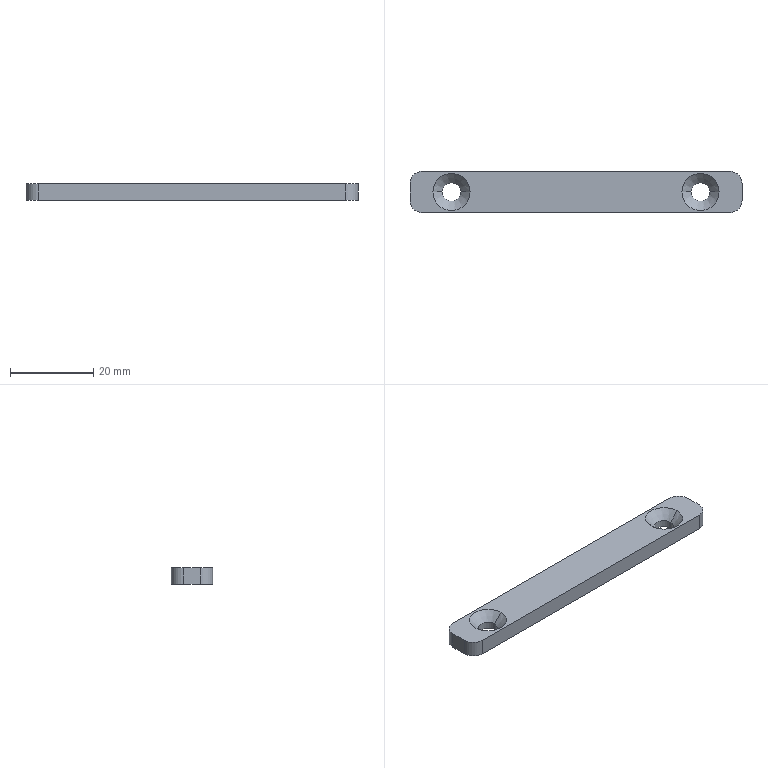Part | STEP file | Belt support strip | 1 solid | 18 faces | box 80 x 10 x 4 mm | volume 2948 mm3 | cylinder 8 | plane 6 | cone 4 | commonest cylinder face diameters 4.5 x4 6 x4
STEP:
#1=CARTESIAN_POINT('',(0.,0.,0.));
#2=DIRECTION('',(0.,0.,1.));
#3=DIRECTION('',(1.,0.,0.));
#4=AXIS2_PLACEMENT_3D('',#1,#2,#3);
#5=CARTESIAN_POINT('',(-116.718,13.068,1.77));
#6=VERTEX_POINT('',#5);
#7=CARTESIAN_POINT('',(-114.488,13.068,4.));
#8=VERTEX_POINT('',#7);
#9=CARTESIAN_POINT('',(-114.488,13.068,4.));
#10=DIRECTION('',(0.7071,0.,0.7071));
#11=VECTOR('',#10,1.);
#12=LINE('',#9,#11);
#13=CARTESIAN_POINT('',(-118.968,13.068,4.));
#14=DIRECTION('',(0.,0.,1.));
#15=DIRECTION('',(1.,0.,0.));
#16=AXIS2_PLACEMENT_3D('',#13,#14,#15);
#17=CONICAL_SURFACE('',#16,4.48,0.7854);
#18=CARTESIAN_POINT('',(6.283,0.));
#19=DIRECTION('',(0.,1.));
#20=VECTOR('',#19,1.);
#21=LINE('',#18,#20);
#22=(GEOMETRIC_REPRESENTATION_CONTEXT(2)PARAMETRIC_REPRESENTATION_CONTEXT()REPRESENTATION_CONTEXT('',''));
#23=DEFINITIONAL_REPRESENTATION('',(#21),#22);
#24=PCURVE('',#17,#23);
#25=CARTESIAN_POINT('',(-118.968,13.068,4.));
#26=DIRECTION('',(0.,0.,1.));
#27=DIRECTION('',(1.,0.,0.));
#28=AXIS2_PLACEMENT_3D('',#25,#26,#27);
#29=CONICAL_SURFACE('',#28,4.48,0.7854);
#30=CARTESIAN_POINT('',(0.,0.));
#31=DIRECTION('',(0.,1.));
#32=VECTOR('',#31,1.);
#33=LINE('',#30,#32);
#34=(GEOMETRIC_REPRESENTATION_CONTEXT(2)PARAMETRIC_REPRESENTATION_CONTEXT()REPRESENTATION_CONTEXT('',''));
#35=DEFINITIONAL_REPRESENTATION('',(#33),#34);
#36=PCURVE('',#29,#35);
#37=SURFACE_CURVE('',#12,(#24,#36),.PCURVE_S1.);
#38=EDGE_CURVE('',#6,#8,#37,.T.);
#39=ORIENTED_EDGE('',*,*,#38,.T.);
#40=CARTESIAN_POINT('',(-123.448,13.068,4.));
#41=VERTEX_POINT('',#40);
#42=CARTESIAN_POINT('',(-118.968,13.068,4.));
#43=DIRECTION('',(0.,0.,1.));
#44=DIRECTION('',(1.,0.,0.));
#45=AXIS2_PLACEMENT_3D('',#42,#43,#44);
#46=CIRCLE('',#45,4.48);
#47=CARTESIAN_POINT('',(0.,0.));
#48=DIRECTION('',(1.,0.));
#49=VECTOR('',#48,1.);
#50=LINE('',#47,#49);
#51=(GEOMETRIC_REPRESENTATION_CONTEXT(2)PARAMETRIC_REPRESENTATION_CONTEXT()REPRESENTATION_CONTEXT('',''));
#52=DEFINITIONAL_REPRESENTATION('',(#50),#51);
#53=PCURVE('',#17,#52);
#54=CARTESIAN_POINT('',(-51.968,15.068,4.));
#55=DIRECTION('',(0.,0.,-1.));
#56=DIRECTION('',(-1.,0.,0.));
#57=AXIS2_PLACEMENT_3D('',#54,#55,#56);
#58=PLANE('',#57);
#59=CARTESIAN_POINT('',(62.52,-2.));
#60=CARTESIAN_POINT('',(62.52,5.76));
#61=CARTESIAN_POINT('',(69.24,1.88));
#62=CARTESIAN_POINT('',(75.96,-2.));
#63=CARTESIAN_POINT('',(69.24,-5.88));
#64=CARTESIAN_POINT('',(62.52,-9.76));
#65=CARTESIAN_POINT('',(62.52,-2.));
#66=(BOUNDED_CURVE()B_SPLINE_CURVE(2,(#59,#60,#61,#62,#63,#64,#65),.UNSPECIFIED.,.T.,.F.)B_SPLINE_CURVE_WITH_KNOTS((1,2,2,2,2,1),(-2.094,0.,2.094,4.189,6.283,8.378),.UNSPECIFIED.)CURVE()GEOMETRIC_REPRESENTATION_ITEM()RATIONAL_B_SPLINE_CURVE((1.,0.5,1.,0.5,1.,0.5,1.))REPRESENTATION_ITEM(''));
#67=(GEOMETRIC_REPRESENTATION_CONTEXT(2)PARAMETRIC_REPRESENTATION_CONTEXT()REPRESENTATION_CONTEXT('',''));
#68=DEFINITIONAL_REPRESENTATION('',(#66),#67);
#69=PCURVE('',#58,#68);
#70=SURFACE_CURVE('',#46,(#53,#69),.PCURVE_S1.);
#71=EDGE_CURVE('',#41,#8,#70,.T.);
#72=ORIENTED_EDGE('',*,*,#71,.F.);
#73=CARTESIAN_POINT('',(-121.218,13.068,1.77));
#74=VERTEX_POINT('',#73);
#75=CARTESIAN_POINT('',(-123.448,13.068,4.));
#76=DIRECTION('',(-0.7071,0.,0.7071));
#77=VECTOR('',#76,1.);
#78=LINE('',#75,#77);
#79=CARTESIAN_POINT('',(3.142,0.));
#80=DIRECTION('',(0.,1.));
#81=VECTOR('',#80,1.);
#82=LINE('',#79,#81);
#83=(GEOMETRIC_REPRESENTATION_CONTEXT(2)PARAMETRIC_REPRESENTATION_CONTEXT()REPRESENTATION_CONTEXT('',''));
#84=DEFINITIONAL_REPRESENTATION('',(#82),#83);
#85=PCURVE('',#17,#84);
#86=CARTESIAN_POINT('',(3.142,0.));
#87=DIRECTION('',(0.,1.));
#88=VECTOR('',#87,1.);
#89=LINE('',#86,#88);
#90=(GEOMETRIC_REPRESENTATION_CONTEXT(2)PARAMETRIC_REPRESENTATION_CONTEXT()REPRESENTATION_CONTEXT('',''));
#91=DEFINITIONAL_REPRESENTATION('',(#89),#90);
#92=PCURVE('',#29,#91);
#93=SURFACE_CURVE('',#78,(#85,#92),.PCURVE_S1.);
#94=EDGE_CURVE('',#74,#41,#93,.T.);
#95=ORIENTED_EDGE('',*,*,#94,.F.);
#96=CARTESIAN_POINT('',(-118.968,13.068,1.77));
#97=DIRECTION('',(0.,0.,1.));
#98=DIRECTION('',(1.,0.,0.));
#99=AXIS2_PLACEMENT_3D('',#96,#97,#98);
#100=CIRCLE('',#99,2.25);
#101=CARTESIAN_POINT('',(0.,-2.23));
#102=DIRECTION('',(1.,0.));
#103=VECTOR('',#102,1.);
#104=LINE('',#101,#103);
#105=(GEOMETRIC_REPRESENTATION_CONTEXT(2)PARAMETRIC_REPRESENTATION_CONTEXT()REPRESENTATION_CONTEXT('',''));
#106=DEFINITIONAL_REPRESENTATION('',(#104),#105);
#107=PCURVE('',#17,#106);
#108=CARTESIAN_POINT('',(-118.968,13.068,4.));
#109=DIRECTION('',(0.,0.,1.));
#110=DIRECTION('',(1.,0.,0.));
#111=AXIS2_PLACEMENT_3D('',#108,#109,#110);
#112=CYLINDRICAL_SURFACE('',#111,2.25);
#113=CARTESIAN_POINT('',(0.,-2.23));
#114=DIRECTION('',(1.,0.));
#115=VECTOR('',#114,1.);
#116=LINE('',#113,#115);
#117=(GEOMETRIC_REPRESENTATION_CONTEXT(2)PARAMETRIC_REPRESENTATION_CONTEXT()REPRESENTATION_CONTEXT('',''));
#118=DEFINITIONAL_REPRESENTATION('',(#116),#117);
#119=PCURVE('',#112,#118);
#120=SURFACE_CURVE('',#100,(#107,#119),.PCURVE_S1.);
#121=EDGE_CURVE('',#74,#6,#120,.T.);
#122=ORIENTED_EDGE('',*,*,#121,.T.);
#123=EDGE_LOOP('',(#39,#72,#95,#122));
#124=FACE_BOUND('',#123,.F.);
#125=ADVANCED_FACE('',(#124),#17,.F.);
#126=CARTESIAN_POINT('',(-116.718,13.068,0.));
#127=VERTEX_POINT('',#126);
#128=CARTESIAN_POINT('',(-116.718,13.068,4.));
#129=DIRECTION('',(0.,0.,1.));
#130=VECTOR('',#129,1.);
#131=LINE('',#128,#130);
#132=CARTESIAN_POINT('',(6.283,0.));
#133=DIRECTION('',(0.,1.));
#134=VECTOR('',#133,1.);
#135=LINE('',#132,#134);
#136=(GEOMETRIC_REPRESENTATION_CONTEXT(2)PARAMETRIC_REPRESENTATION_CONTEXT()REPRESENTATION_CONTEXT('',''));
#137=DEFINITIONAL_REPRESENTATION('',(#135),#136);
#138=PCURVE('',#112,#137);
#139=CARTESIAN_POINT('',(-118.968,13.068,4.));
#140=DIRECTION('',(0.,0.,1.));
#141=DIRECTION('',(1.,0.,0.));
#142=AXIS2_PLACEMENT_3D('',#139,#140,#141);
#143=CYLINDRICAL_SURFACE('',#142,2.25);
#144=CARTESIAN_POINT('',(0.,0.));
#145=DIRECTION('',(0.,1.));
#146=VECTOR('',#145,1.);
#147=LINE('',#144,#146);
#148=(GEOMETRIC_REPRESENTATION_CONTEXT(2)PARAMETRIC_REPRESENTATION_CONTEXT()REPRESENTATION_CONTEXT('',''));
#149=DEFINITIONAL_REPRESENTATION('',(#147),#148);
#150=PCURVE('',#143,#149);
#151=SURFACE_CURVE('',#131,(#138,#150),.PCURVE_S1.);
#152=EDGE_CURVE('',#127,#6,#151,.T.);
#153=ORIENTED_EDGE('',*,*,#152,.T.);
#154=ORIENTED_EDGE('',*,*,#121,.F.);
#155=CARTESIAN_POINT('',(-121.218,13.068,0.));
#156=VERTEX_POINT('',#155);
#157=CARTESIAN_POINT('',(-121.218,13.068,4.));
#158=DIRECTION('',(0.,0.,1.));
#159=VECTOR('',#158,1.);
#160=LINE('',#157,#159);
#161=CARTESIAN_POINT('',(3.142,0.));
#162=DIRECTION('',(0.,1.));
#163=VECTOR('',#162,1.);
#164=LINE('',#161,#163);
#165=(GEOMETRIC_REPRESENTATION_CONTEXT(2)PARAMETRIC_REPRESENTATION_CONTEXT()REPRESENTATION_CONTEXT('',''));
#166=DEFINITIONAL_REPRESENTATION('',(#164),#165);
#167=PCURVE('',#112,#166);
#168=CARTESIAN_POINT('',(3.142,0.));
#169=DIRECTION('',(0.,1.));
#170=VECTOR('',#169,1.);
#171=LINE('',#168,#170);
#172=(GEOMETRIC_REPRESENTATION_CONTEXT(2)PARAMETRIC_REPRESENTATION_CONTEXT()REPRESENTATION_CONTEXT('',''));
#173=DEFINITIONAL_REPRESENTATION('',(#171),#172);
#174=PCURVE('',#143,#173);
#175=SURFACE_CURVE('',#160,(#167,#174),.PCURVE_S1.);
#176=EDGE_CURVE('',#156,#74,#175,.T.);
#177=ORIENTED_EDGE('',*,*,#176,.F.);
#178=CARTESIAN_POINT('',(-118.968,13.068,0.));
#179=DIRECTION('',(0.,0.,1.));
#180=DIRECTION('',(1.,0.,0.));
#181=AXIS2_PLACEMENT_3D('',#178,#179,#180);
#182=CIRCLE('',#181,2.25);
#183=CARTESIAN_POINT('',(0.,-4.));
#184=DIRECTION('',(1.,0.));
#185=VECTOR('',#184,1.);
#186=LINE('',#183,#185);
#187=(GEOMETRIC_REPRESENTATION_CONTEXT(2)PARAMETRIC_REPRESENTATION_CONTEXT()REPRESENTATION_CONTEXT('',''));
#188=DEFINITIONAL_REPRESENTATION('',(#186),#187);
#189=PCURVE('',#112,#188);
#190=CARTESIAN_POINT('',(-51.968,15.068,0.));
#191=DIRECTION('',(0.,0.,-1.));
#192=DIRECTION('',(-1.,0.,0.));
#193=AXIS2_PLACEMENT_3D('',#190,#191,#192);
#194=PLANE('',#193);
#195=CARTESIAN_POINT('',(64.75,-2.));
#196=CARTESIAN_POINT('',(64.75,1.897));
#197=CARTESIAN_POINT('',(68.125,-0.05144));
#198=CARTESIAN_POINT('',(71.5,-2.));
#199=CARTESIAN_POINT('',(68.125,-3.949));
#200=CARTESIAN_POINT('',(64.75,-5.897));
#201=CARTESIAN_POINT('',(64.75,-2.));
#202=(BOUNDED_CURVE()B_SPLINE_CURVE(2,(#195,#196,#197,#198,#199,#200,#201),.UNSPECIFIED.,.T.,.F.)B_SPLINE_CURVE_WITH_KNOTS((1,2,2,2,2,1),(-2.094,0.,2.094,4.189,6.283,8.378),.UNSPECIFIED.)CURVE()GEOMETRIC_REPRESENTATION_ITEM()RATIONAL_B_SPLINE_CURVE((1.,0.5,1.,0.5,1.,0.5,1.))REPRESENTATION_ITEM(''));
#203=(GEOMETRIC_REPRESENTATION_CONTEXT(2)PARAMETRIC_REPRESENTATION_CONTEXT()REPRESENTATION_CONTEXT('',''));
#204=DEFINITIONAL_REPRESENTATION('',(#202),#203);
#205=PCURVE('',#194,#204);
#206=SURFACE_CURVE('',#182,(#189,#205),.PCURVE_S1.);
#207=EDGE_CURVE('',#156,#127,#206,.T.);
#208=ORIENTED_EDGE('',*,*,#207,.T.);
#209=EDGE_LOOP('',(#153,#154,#177,#208));
#210=FACE_BOUND('',#209,.F.);
#211=ADVANCED_FACE('',(#210),#112,.F.);
#212=CARTESIAN_POINT('',(-56.718,13.068,1.77));
#213=VERTEX_POINT('',#212);
#214=CARTESIAN_POINT('',(-54.488,13.068,4.));
#215=VERTEX_POINT('',#214);
#216=CARTESIAN_POINT('',(-54.488,13.068,4.));
#217=DIRECTION('',(0.7071,0.,0.7071));
#218=VECTOR('',#217,1.);
#219=LINE('',#216,#218);
#220=CARTESIAN_POINT('',(-58.968,13.068,4.));
#221=DIRECTION('',(0.,0.,1.));
#222=DIRECTION('',(1.,0.,0.));
#223=AXIS2_PLACEMENT_3D('',#220,#221,#222);
#224=CONICAL_SURFACE('',#223,4.48,0.7854);
#225=CARTESIAN_POINT('',(6.283,0.));
#226=DIRECTION('',(0.,1.));
#227=VECTOR('',#226,1.);
#228=LINE('',#225,#227);
#229=(GEOMETRIC_REPRESENTATION_CONTEXT(2)PARAMETRIC_REPRESENTATION_CONTEXT()REPRESENTATION_CONTEXT('',''));
#230=DEFINITIONAL_REPRESENTATION('',(#228),#229);
#231=PCURVE('',#224,#230);
#232=CARTESIAN_POINT('',(-58.968,13.068,4.));
#233=DIRECTION('',(0.,0.,1.));
#234=DIRECTION('',(1.,0.,0.));
#235=AXIS2_PLACEMENT_3D('',#232,#233,#234);
#236=CONICAL_SURFACE('',#235,4.48,0.7854);
#237=CARTESIAN_POINT('',(0.,0.));
#238=DIRECTION('',(0.,1.));
#239=VECTOR('',#238,1.);
#240=LINE('',#237,#239);
#241=(GEOMETRIC_REPRESENTATION_CONTEXT(2)PARAMETRIC_REPRESENTATION_CONTEXT()REPRESENTATION_CONTEXT('',''));
#242=DEFINITIONAL_REPRESENTATION('',(#240),#241);
#243=PCURVE('',#236,#242);
#244=SURFACE_CURVE('',#219,(#231,#243),.PCURVE_S1.);
#245=EDGE_CURVE('',#213,#215,#244,.T.);
#246=ORIENTED_EDGE('',*,*,#245,.T.);
#247=CARTESIAN_POINT('',(-63.448,13.068,4.));
#248=VERTEX_POINT('',#247);
#249=CARTESIAN_POINT('',(-58.968,13.068,4.));
#250=DIRECTION('',(0.,0.,1.));
#251=DIRECTION('',(1.,0.,0.));
#252=AXIS2_PLACEMENT_3D('',#249,#250,#251);
#253=CIRCLE('',#252,4.48);
#254=CARTESIAN_POINT('',(0.,0.));
#255=DIRECTION('',(1.,0.));
#256=VECTOR('',#255,1.);
#257=LINE('',#254,#256);
#258=(GEOMETRIC_REPRESENTATION_CONTEXT(2)PARAMETRIC_REPRESENTATION_CONTEXT()REPRESENTATION_CONTEXT('',''));
#259=DEFINITIONAL_REPRESENTATION('',(#257),#258);
#260=PCURVE('',#224,#259);
#261=CARTESIAN_POINT('',(2.52,-2.));
#262=CARTESIAN_POINT('',(2.52,5.76));
#263=CARTESIAN_POINT('',(9.24,1.88));
#264=CARTESIAN_POINT('',(15.96,-2.));
#265=CARTESIAN_POINT('',(9.24,-5.88));
#266=CARTESIAN_POINT('',(2.52,-9.76));
#267=CARTESIAN_POINT('',(2.52,-2.));
#268=(BOUNDED_CURVE()B_SPLINE_CURVE(2,(#261,#262,#263,#264,#265,#266,#267),.UNSPECIFIED.,.T.,.F.)B_SPLINE_CURVE_WITH_KNOTS((1,2,2,2,2,1),(-2.094,0.,2.094,4.189,6.283,8.378),.UNSPECIFIED.)CURVE()GEOMETRIC_REPRESENTATION_ITEM()RATIONAL_B_SPLINE_CURVE((1.,0.5,1.,0.5,1.,0.5,1.))REPRESENTATION_ITEM(''));
#269=(GEOMETRIC_REPRESENTATION_CONTEXT(2)PARAMETRIC_REPRESENTATION_CONTEXT()REPRESENTATION_CONTEXT('',''));
#270=DEFINITIONAL_REPRESENTATION('',(#268),#269);
#271=PCURVE('',#58,#270);
#272=SURFACE_CURVE('',#253,(#260,#271),.PCURVE_S1.);
#273=EDGE_CURVE('',#248,#215,#272,.T.);
#274=ORIENTED_EDGE('',*,*,#273,.F.);
#275=CARTESIAN_POINT('',(-61.218,13.068,1.77));
#276=VERTEX_POINT('',#275);
#277=CARTESIAN_POINT('',(-63.448,13.068,4.));
#278=DIRECTION('',(-0.7071,0.,0.7071));
#279=VECTOR('',#278,1.);
#280=LINE('',#277,#279);
#281=CARTESIAN_POINT('',(3.142,0.));
#282=DIRECTION('',(0.,1.));
#283=VECTOR('',#282,1.);
#284=LINE('',#281,#283);
#285=(GEOMETRIC_REPRESENTATION_CONTEXT(2)PARAMETRIC_REPRESENTATION_CONTEXT()REPRESENTATION_CONTEXT('',''));
#286=DEFINITIONAL_REPRESENTATION('',(#284),#285);
#287=PCURVE('',#224,#286);
#288=CARTESIAN_POINT('',(3.142,0.));
#289=DIRECTION('',(0.,1.));
#290=VECTOR('',#289,1.);
#291=LINE('',#288,#290);
#292=(GEOMETRIC_REPRESENTATION_CONTEXT(2)PARAMETRIC_REPRESENTATION_CONTEXT()REPRESENTATION_CONTEXT('',''));
#293=DEFINITIONAL_REPRESENTATION('',(#291),#292);
#294=PCURVE('',#236,#293);
#295=SURFACE_CURVE('',#280,(#287,#294),.PCURVE_S1.);
#296=EDGE_CURVE('',#276,#248,#295,.T.);
#297=ORIENTED_EDGE('',*,*,#296,.F.);
#298=CARTESIAN_POINT('',(-58.968,13.068,1.77));
#299=DIRECTION('',(0.,0.,1.));
#300=DIRECTION('',(1.,0.,0.));
#301=AXIS2_PLACEMENT_3D('',#298,#299,#300);
#302=CIRCLE('',#301,2.25);
#303=CARTESIAN_POINT('',(0.,-2.23));
#304=DIRECTION('',(1.,0.));
#305=VECTOR('',#304,1.);
#306=LINE('',#303,#305);
#307=(GEOMETRIC_REPRESENTATION_CONTEXT(2)PARAMETRIC_REPRESENTATION_CONTEXT()REPRESENTATION_CONTEXT('',''));
#308=DEFINITIONAL_REPRESENTATION('',(#306),#307);
#309=PCURVE('',#224,#308);
#310=CARTESIAN_POINT('',(-58.968,13.068,4.));
#311=DIRECTION('',(0.,0.,1.));
#312=DIRECTION('',(1.,0.,0.));
#313=AXIS2_PLACEMENT_3D('',#310,#311,#312);
#314=CYLINDRICAL_SURFACE('',#313,2.25);
#315=CARTESIAN_POINT('',(0.,-2.23));
#316=DIRECTION('',(1.,0.));
#317=VECTOR('',#316,1.);
#318=LINE('',#315,#317);
#319=(GEOMETRIC_REPRESENTATION_CONTEXT(2)PARAMETRIC_REPRESENTATION_CONTEXT()REPRESENTATION_CONTEXT('',''));
#320=DEFINITIONAL_REPRESENTATION('',(#318),#319);
#321=PCURVE('',#314,#320);
#322=SURFACE_CURVE('',#302,(#309,#321),.PCURVE_S1.);
#323=EDGE_CURVE('',#276,#213,#322,.T.);
#324=ORIENTED_EDGE('',*,*,#323,.T.);
#325=EDGE_LOOP('',(#246,#274,#297,#324));
#326=FACE_BOUND('',#325,.F.);
#327=ADVANCED_FACE('',(#326),#224,.F.);
#328=CARTESIAN_POINT('',(-56.718,13.068,0.));
#329=VERTEX_POINT('',#328);
#330=CARTESIAN_POINT('',(-56.718,13.068,4.));
#331=DIRECTION('',(0.,0.,1.));
#332=VECTOR('',#331,1.);
#333=LINE('',#330,#332);
#334=CARTESIAN_POINT('',(6.283,0.));
#335=DIRECTION('',(0.,1.));
#336=VECTOR('',#335,1.);
#337=LINE('',#334,#336);
#338=(GEOMETRIC_REPRESENTATION_CONTEXT(2)PARAMETRIC_REPRESENTATION_CONTEXT()REPRESENTATION_CONTEXT('',''));
#339=DEFINITIONAL_REPRESENTATION('',(#337),#338);
#340=PCURVE('',#314,#339);
#341=CARTESIAN_POINT('',(-58.968,13.068,4.));
#342=DIRECTION('',(0.,0.,1.));
#343=DIRECTION('',(1.,0.,0.));
#344=AXIS2_PLACEMENT_3D('',#341,#342,#343);
#345=CYLINDRICAL_SURFACE('',#344,2.25);
#346=CARTESIAN_POINT('',(0.,0.));
#347=DIRECTION('',(0.,1.));
#348=VECTOR('',#347,1.);
#349=LINE('',#346,#348);
#350=(GEOMETRIC_REPRESENTATION_CONTEXT(2)PARAMETRIC_REPRESENTATION_CONTEXT()REPRESENTATION_CONTEXT('',''));
#351=DEFINITIONAL_REPRESENTATION('',(#349),#350);
#352=PCURVE('',#345,#351);
#353=SURFACE_CURVE('',#333,(#340,#352),.PCURVE_S1.);
#354=EDGE_CURVE('',#329,#213,#353,.T.);
#355=ORIENTED_EDGE('',*,*,#354,.T.);
#356=ORIENTED_EDGE('',*,*,#323,.F.);
#357=CARTESIAN_POINT('',(-61.218,13.068,0.));
#358=VERTEX_POINT('',#357);
#359=CARTESIAN_POINT('',(-61.218,13.068,4.));
#360=DIRECTION('',(0.,0.,1.));
#361=VECTOR('',#360,1.);
#362=LINE('',#359,#361);
#363=CARTESIAN_POINT('',(3.142,0.));
#364=DIRECTION('',(0.,1.));
#365=VECTOR('',#364,1.);
#366=LINE('',#363,#365);
#367=(GEOMETRIC_REPRESENTATION_CONTEXT(2)PARAMETRIC_REPRESENTATION_CONTEXT()REPRESENTATION_CONTEXT('',''));
#368=DEFINITIONAL_REPRESENTATION('',(#366),#367);
#369=PCURVE('',#314,#368);
#370=CARTESIAN_POINT('',(3.142,0.));
#371=DIRECTION('',(0.,1.));
#372=VECTOR('',#371,1.);
#373=LINE('',#370,#372);
#374=(GEOMETRIC_REPRESENTATION_CONTEXT(2)PARAMETRIC_REPRESENTATION_CONTEXT()REPRESENTATION_CONTEXT('',''));
#375=DEFINITIONAL_REPRESENTATION('',(#373),#374);
#376=PCURVE('',#345,#375);
#377=SURFACE_CURVE('',#362,(#369,#376),.PCURVE_S1.);
#378=EDGE_CURVE('',#358,#276,#377,.T.);
#379=ORIENTED_EDGE('',*,*,#378,.F.);
#380=CARTESIAN_POINT('',(-58.968,13.068,0.));
#381=DIRECTION('',(0.,0.,1.));
#382=DIRECTION('',(1.,0.,0.));
#383=AXIS2_PLACEMENT_3D('',#380,#381,#382);
#384=CIRCLE('',#383,2.25);
#385=CARTESIAN_POINT('',(0.,-4.));
#386=DIRECTION('',(1.,0.));
#387=VECTOR('',#386,1.);
#388=LINE('',#385,#387);
#389=(GEOMETRIC_REPRESENTATION_CONTEXT(2)PARAMETRIC_REPRESENTATION_CONTEXT()REPRESENTATION_CONTEXT('',''));
#390=DEFINITIONAL_REPRESENTATION('',(#388),#389);
#391=PCURVE('',#314,#390);
#392=CARTESIAN_POINT('',(4.75,-2.));
#393=CARTESIAN_POINT('',(4.75,1.897));
#394=CARTESIAN_POINT('',(8.125,-0.05144));
#395=CARTESIAN_POINT('',(11.5,-2.));
#396=CARTESIAN_POINT('',(8.125,-3.949));
#397=CARTESIAN_POINT('',(4.75,-5.897));
#398=CARTESIAN_POINT('',(4.75,-2.));
#399=(BOUNDED_CURVE()B_SPLINE_CURVE(2,(#392,#393,#394,#395,#396,#397,#398),.UNSPECIFIED.,.T.,.F.)B_SPLINE_CURVE_WITH_KNOTS((1,2,2,2,2,1),(-2.094,0.,2.094,4.189,6.283,8.378),.UNSPECIFIED.)CURVE()GEOMETRIC_REPRESENTATION_ITEM()RATIONAL_B_SPLINE_CURVE((1.,0.5,1.,0.5,1.,0.5,1.))REPRESENTATION_ITEM(''));
#400=(GEOMETRIC_REPRESENTATION_CONTEXT(2)PARAMETRIC_REPRESENTATION_CONTEXT()REPRESENTATION_CONTEXT('',''));
#401=DEFINITIONAL_REPRESENTATION('',(#399),#400);
#402=PCURVE('',#194,#401);
#403=SURFACE_CURVE('',#384,(#391,#402),.PCURVE_S1.);
#404=EDGE_CURVE('',#358,#329,#403,.T.);
#405=ORIENTED_EDGE('',*,*,#404,.T.);
#406=EDGE_LOOP('',(#355,#356,#379,#405));
#407=FACE_BOUND('',#406,.F.);
#408=ADVANCED_FACE('',(#407),#314,.F.);
#409=CARTESIAN_POINT('',(-118.968,13.068,4.));
#410=DIRECTION('',(0.,0.,1.));
#411=DIRECTION('',(1.,0.,0.));
#412=AXIS2_PLACEMENT_3D('',#409,#410,#411);
#413=CIRCLE('',#412,4.48);
#414=CARTESIAN_POINT('',(62.52,-2.));
#415=CARTESIAN_POINT('',(62.52,5.76));
#416=CARTESIAN_POINT('',(69.24,1.88));
#417=CARTESIAN_POINT('',(75.96,-2.));
#418=CARTESIAN_POINT('',(69.24,-5.88));
#419=CARTESIAN_POINT('',(62.52,-9.76));
#420=CARTESIAN_POINT('',(62.52,-2.));
#421=(BOUNDED_CURVE()B_SPLINE_CURVE(2,(#414,#415,#416,#417,#418,#419,#420),.UNSPECIFIED.,.T.,.F.)B_SPLINE_CURVE_WITH_KNOTS((1,2,2,2,2,1),(-2.094,0.,2.094,4.189,6.283,8.378),.UNSPECIFIED.)CURVE()GEOMETRIC_REPRESENTATION_ITEM()RATIONAL_B_SPLINE_CURVE((1.,0.5,1.,0.5,1.,0.5,1.))REPRESENTATION_ITEM(''));
#422=(GEOMETRIC_REPRESENTATION_CONTEXT(2)PARAMETRIC_REPRESENTATION_CONTEXT()REPRESENTATION_CONTEXT('',''));
#423=DEFINITIONAL_REPRESENTATION('',(#421),#422);
#424=PCURVE('',#58,#423);
#425=CARTESIAN_POINT('',(0.,0.));
#426=DIRECTION('',(1.,0.));
#427=VECTOR('',#426,1.);
#428=LINE('',#425,#427);
#429=(GEOMETRIC_REPRESENTATION_CONTEXT(2)PARAMETRIC_REPRESENTATION_CONTEXT()REPRESENTATION_CONTEXT('',''));
#430=DEFINITIONAL_REPRESENTATION('',(#428),#429);
#431=PCURVE('',#29,#430);
#432=SURFACE_CURVE('',#413,(#424,#431),.PCURVE_S1.);
#433=EDGE_CURVE('',#8,#41,#432,.T.);
#434=ORIENTED_EDGE('',*,*,#433,.F.);
#435=ORIENTED_EDGE('',*,*,#71,.F.);
#436=EDGE_LOOP('',(#434,#435));
#437=FACE_BOUND('',#436,.T.);
#438=CARTESIAN_POINT('',(-58.968,13.068,4.));
#439=DIRECTION('',(0.,0.,1.));
#440=DIRECTION('',(1.,0.,0.));
#441=AXIS2_PLACEMENT_3D('',#438,#439,#440);
#442=CIRCLE('',#441,4.48);
#443=CARTESIAN_POINT('',(2.52,-2.));
#444=CARTESIAN_POINT('',(2.52,5.76));
#445=CARTESIAN_POINT('',(9.24,1.88));
#446=CARTESIAN_POINT('',(15.96,-2.));
#447=CARTESIAN_POINT('',(9.24,-5.88));
#448=CARTESIAN_POINT('',(2.52,-9.76));
#449=CARTESIAN_POINT('',(2.52,-2.));
#450=(BOUNDED_CURVE()B_SPLINE_CURVE(2,(#443,#444,#445,#446,#447,#448,#449),.UNSPECIFIED.,.T.,.F.)B_SPLINE_CURVE_WITH_KNOTS((1,2,2,2,2,1),(-2.094,0.,2.094,4.189,6.283,8.378),.UNSPECIFIED.)CURVE()GEOMETRIC_REPRESENTATION_ITEM()RATIONAL_B_SPLINE_CURVE((1.,0.5,1.,0.5,1.,0.5,1.))REPRESENTATION_ITEM(''));
#451=(GEOMETRIC_REPRESENTATION_CONTEXT(2)PARAMETRIC_REPRESENTATION_CONTEXT()REPRESENTATION_CONTEXT('',''));
#452=DEFINITIONAL_REPRESENTATION('',(#450),#451);
#453=PCURVE('',#58,#452);
#454=CARTESIAN_POINT('',(0.,0.));
#455=DIRECTION('',(1.,0.));
#456=VECTOR('',#455,1.);
#457=LINE('',#454,#456);
#458=(GEOMETRIC_REPRESENTATION_CONTEXT(2)PARAMETRIC_REPRESENTATION_CONTEXT()REPRESENTATION_CONTEXT('',''));
#459=DEFINITIONAL_REPRESENTATION('',(#457),#458);
#460=PCURVE('',#236,#459);
#461=SURFACE_CURVE('',#442,(#453,#460),.PCURVE_S1.);
#462=EDGE_CURVE('',#215,#248,#461,.T.);
#463=ORIENTED_EDGE('',*,*,#462,.F.);
#464=ORIENTED_EDGE('',*,*,#273,.F.);
#465=EDGE_LOOP('',(#463,#464));
#466=FACE_BOUND('',#465,.T.);
#467=CARTESIAN_POINT('',(-48.968,15.068,4.));
#468=VERTEX_POINT('',#467);
#469=CARTESIAN_POINT('',(-51.968,18.068,4.));
#470=VERTEX_POINT('',#469);
#471=CARTESIAN_POINT('',(-51.968,15.068,4.));
#472=DIRECTION('',(0.,0.,1.));
#473=DIRECTION('',(-1.,0.,0.));
#474=AXIS2_PLACEMENT_3D('',#471,#472,#473);
#475=CIRCLE('',#474,3.);
#476=CARTESIAN_POINT('',(3.,0.));
#477=CARTESIAN_POINT('',(3.,-5.196));
#478=CARTESIAN_POINT('',(-1.5,-2.598));
#479=CARTESIAN_POINT('',(-6.,0.));
#480=CARTESIAN_POINT('',(-1.5,2.598));
#481=CARTESIAN_POINT('',(3.,5.196));
#482=CARTESIAN_POINT('',(3.,0.));
#483=(BOUNDED_CURVE()B_SPLINE_CURVE(2,(#476,#477,#478,#479,#480,#481,#482),.UNSPECIFIED.,.T.,.F.)B_SPLINE_CURVE_WITH_KNOTS((1,2,2,2,2,1),(-2.094,0.,2.094,4.189,6.283,8.378),.UNSPECIFIED.)CURVE()GEOMETRIC_REPRESENTATION_ITEM()RATIONAL_B_SPLINE_CURVE((1.,0.5,1.,0.5,1.,0.5,1.))REPRESENTATION_ITEM(''));
#484=(GEOMETRIC_REPRESENTATION_CONTEXT(2)PARAMETRIC_REPRESENTATION_CONTEXT()REPRESENTATION_CONTEXT('',''));
#485=DEFINITIONAL_REPRESENTATION('',(#483),#484);
#486=PCURVE('',#58,#485);
#487=CARTESIAN_POINT('',(-51.968,15.068,4.));
#488=DIRECTION('',(0.,0.,-1.));
#489=DIRECTION('',(-1.,0.,0.));
#490=AXIS2_PLACEMENT_3D('',#487,#488,#489);
#491=CYLINDRICAL_SURFACE('',#490,3.);
#492=CARTESIAN_POINT('',(6.283,0.));
#493=DIRECTION('',(-1.,0.));
#494=VECTOR('',#493,1.);
#495=LINE('',#492,#494);
#496=(GEOMETRIC_REPRESENTATION_CONTEXT(2)PARAMETRIC_REPRESENTATION_CONTEXT()REPRESENTATION_CONTEXT('',''));
#497=DEFINITIONAL_REPRESENTATION('',(#495),#496);
#498=PCURVE('',#491,#497);
#499=SURFACE_CURVE('',#475,(#486,#498),.PCURVE_S1.);
#500=EDGE_CURVE('',#468,#470,#499,.T.);
#501=ORIENTED_EDGE('',*,*,#500,.T.);
#502=CARTESIAN_POINT('',(-125.968,18.068,4.));
#503=VERTEX_POINT('',#502);
#504=CARTESIAN_POINT('',(-125.968,18.068,4.));
#505=DIRECTION('',(-1.,0.,0.));
#506=VECTOR('',#505,1.);
#507=LINE('',#504,#506);
#508=CARTESIAN_POINT('',(74.,3.));
#509=DIRECTION('',(1.,0.));
#510=VECTOR('',#509,1.);
#511=LINE('',#508,#510);
#512=(GEOMETRIC_REPRESENTATION_CONTEXT(2)PARAMETRIC_REPRESENTATION_CONTEXT()REPRESENTATION_CONTEXT('',''));
#513=DEFINITIONAL_REPRESENTATION('',(#511),#512);
#514=PCURVE('',#58,#513);
#515=CARTESIAN_POINT('',(-125.968,18.068,4.));
#516=DIRECTION('',(0.,-1.,0.));
#517=DIRECTION('',(0.,0.,-1.));
#518=AXIS2_PLACEMENT_3D('',#515,#516,#517);
#519=PLANE('',#518);
#520=CARTESIAN_POINT('',(0.,0.));
#521=DIRECTION('',(0.,-1.));
#522=VECTOR('',#521,1.);
#523=LINE('',#520,#522);
#524=(GEOMETRIC_REPRESENTATION_CONTEXT(2)PARAMETRIC_REPRESENTATION_CONTEXT()REPRESENTATION_CONTEXT('',''));
#525=DEFINITIONAL_REPRESENTATION('',(#523),#524);
#526=PCURVE('',#519,#525);
#527=SURFACE_CURVE('',#507,(#514,#526),.PCURVE_S1.);
#528=EDGE_CURVE('',#470,#503,#527,.T.);
#529=ORIENTED_EDGE('',*,*,#528,.T.);
#530=CARTESIAN_POINT('',(-128.968,15.068,4.));
#531=VERTEX_POINT('',#530);
#532=CARTESIAN_POINT('',(-125.968,15.068,4.));
#533=DIRECTION('',(0.,0.,1.));
#534=DIRECTION('',(1.,0.,0.));
#535=AXIS2_PLACEMENT_3D('',#532,#533,#534);
#536=CIRCLE('',#535,3.);
#537=CARTESIAN_POINT('',(71.,0.));
#538=CARTESIAN_POINT('',(71.,5.196));
#539=CARTESIAN_POINT('',(75.5,2.598));
#540=CARTESIAN_POINT('',(80.,0.));
#541=CARTESIAN_POINT('',(75.5,-2.598));
#542=CARTESIAN_POINT('',(71.,-5.196));
#543=CARTESIAN_POINT('',(71.,0.));
#544=(BOUNDED_CURVE()B_SPLINE_CURVE(2,(#537,#538,#539,#540,#541,#542,#543),.UNSPECIFIED.,.T.,.F.)B_SPLINE_CURVE_WITH_KNOTS((1,2,2,2,2,1),(-2.094,0.,2.094,4.189,6.283,8.378),.UNSPECIFIED.)CURVE()GEOMETRIC_REPRESENTATION_ITEM()RATIONAL_B_SPLINE_CURVE((1.,0.5,1.,0.5,1.,0.5,1.))REPRESENTATION_ITEM(''));
#545=(GEOMETRIC_REPRESENTATION_CONTEXT(2)PARAMETRIC_REPRESENTATION_CONTEXT()REPRESENTATION_CONTEXT('',''));
#546=DEFINITIONAL_REPRESENTATION('',(#544),#545);
#547=PCURVE('',#58,#546);
#548=CARTESIAN_POINT('',(-125.968,15.068,4.));
#549=DIRECTION('',(0.,0.,-1.));
#550=DIRECTION('',(-1.,0.,0.));
#551=AXIS2_PLACEMENT_3D('',#548,#549,#550);
#552=CYLINDRICAL_SURFACE('',#551,3.);
#553=CARTESIAN_POINT('',(3.142,0.));
#554=DIRECTION('',(-1.,0.));
#555=VECTOR('',#554,1.);
#556=LINE('',#553,#555);
#557=(GEOMETRIC_REPRESENTATION_CONTEXT(2)PARAMETRIC_REPRESENTATION_CONTEXT()REPRESENTATION_CONTEXT('',''));
#558=DEFINITIONAL_REPRESENTATION('',(#556),#557);
#559=PCURVE('',#552,#558);
#560=SURFACE_CURVE('',#536,(#547,#559),.PCURVE_S1.);
#561=EDGE_CURVE('',#503,#531,#560,.T.);
#562=ORIENTED_EDGE('',*,*,#561,.T.);
#563=CARTESIAN_POINT('',(-128.968,11.068,4.));
#564=VERTEX_POINT('',#563);
#565=CARTESIAN_POINT('',(-128.968,11.068,4.));
#566=DIRECTION('',(0.,-1.,0.));
#567=VECTOR('',#566,1.);
#568=LINE('',#565,#567);
#569=CARTESIAN_POINT('',(77.,-4.));
#570=DIRECTION('',(0.,-1.));
#571=VECTOR('',#570,1.);
#572=LINE('',#569,#571);
#573=(GEOMETRIC_REPRESENTATION_CONTEXT(2)PARAMETRIC_REPRESENTATION_CONTEXT()REPRESENTATION_CONTEXT('',''));
#574=DEFINITIONAL_REPRESENTATION('',(#572),#573);
#575=PCURVE('',#58,#574);
#576=CARTESIAN_POINT('',(-128.968,11.068,4.));
#577=DIRECTION('',(1.,0.,0.));
#578=DIRECTION('',(0.,0.,-1.));
#579=AXIS2_PLACEMENT_3D('',#576,#577,#578);
#580=PLANE('',#579);
#581=CARTESIAN_POINT('',(0.,0.));
#582=DIRECTION('',(0.,-1.));
#583=VECTOR('',#582,1.);
#584=LINE('',#581,#583);
#585=(GEOMETRIC_REPRESENTATION_CONTEXT(2)PARAMETRIC_REPRESENTATION_CONTEXT()REPRESENTATION_CONTEXT('',''));
#586=DEFINITIONAL_REPRESENTATION('',(#584),#585);
#587=PCURVE('',#580,#586);
#588=SURFACE_CURVE('',#568,(#575,#587),.PCURVE_S1.);
#589=EDGE_CURVE('',#531,#564,#588,.T.);
#590=ORIENTED_EDGE('',*,*,#589,.T.);
#591=CARTESIAN_POINT('',(-125.968,8.068,4.));
#592=VERTEX_POINT('',#591);
#593=CARTESIAN_POINT('',(-125.968,11.068,4.));
#594=DIRECTION('',(0.,0.,1.));
#595=DIRECTION('',(1.,0.,0.));
#596=AXIS2_PLACEMENT_3D('',#593,#594,#595);
#597=CIRCLE('',#596,3.);
#598=CARTESIAN_POINT('',(71.,-4.));
#599=CARTESIAN_POINT('',(71.,1.196));
#600=CARTESIAN_POINT('',(75.5,-1.402));
#601=CARTESIAN_POINT('',(80.,-4.));
#602=CARTESIAN_POINT('',(75.5,-6.598));
#603=CARTESIAN_POINT('',(71.,-9.196));
#604=CARTESIAN_POINT('',(71.,-4.));
#605=(BOUNDED_CURVE()B_SPLINE_CURVE(2,(#598,#599,#600,#601,#602,#603,#604),.UNSPECIFIED.,.T.,.F.)B_SPLINE_CURVE_WITH_KNOTS((1,2,2,2,2,1),(-2.094,0.,2.094,4.189,6.283,8.378),.UNSPECIFIED.)CURVE()GEOMETRIC_REPRESENTATION_ITEM()RATIONAL_B_SPLINE_CURVE((1.,0.5,1.,0.5,1.,0.5,1.))REPRESENTATION_ITEM(''));
#606=(GEOMETRIC_REPRESENTATION_CONTEXT(2)PARAMETRIC_REPRESENTATION_CONTEXT()REPRESENTATION_CONTEXT('',''));
#607=DEFINITIONAL_REPRESENTATION('',(#605),#606);
#608=PCURVE('',#58,#607);
#609=CARTESIAN_POINT('',(-125.968,11.068,4.));
#610=DIRECTION('',(0.,0.,-1.));
#611=DIRECTION('',(-1.,0.,0.));
#612=AXIS2_PLACEMENT_3D('',#609,#610,#611);
#613=CYLINDRICAL_SURFACE('',#612,3.);
#614=CARTESIAN_POINT('',(9.425,0.));
#615=DIRECTION('',(-1.,0.));
#616=VECTOR('',#615,1.);
#617=LINE('',#614,#616);
#618=(GEOMETRIC_REPRESENTATION_CONTEXT(2)PARAMETRIC_REPRESENTATION_CONTEXT()REPRESENTATION_CONTEXT('',''));
#619=DEFINITIONAL_REPRESENTATION('',(#617),#618);
#620=PCURVE('',#613,#619);
#621=SURFACE_CURVE('',#597,(#608,#620),.PCURVE_S1.);
#622=EDGE_CURVE('',#564,#592,#621,.T.);
#623=ORIENTED_EDGE('',*,*,#622,.T.);
#624=CARTESIAN_POINT('',(-51.968,8.068,4.));
#625=VERTEX_POINT('',#624);
#626=CARTESIAN_POINT('',(-125.968,8.068,4.));
#627=DIRECTION('',(1.,0.,0.));
#628=VECTOR('',#627,1.);
#629=LINE('',#626,#628);
#630=CARTESIAN_POINT('',(74.,-7.));
#631=DIRECTION('',(-1.,0.));
#632=VECTOR('',#631,1.);
#633=LINE('',#630,#632);
#634=(GEOMETRIC_REPRESENTATION_CONTEXT(2)PARAMETRIC_REPRESENTATION_CONTEXT()REPRESENTATION_CONTEXT('',''));
#635=DEFINITIONAL_REPRESENTATION('',(#633),#634);
#636=PCURVE('',#58,#635);
#637=CARTESIAN_POINT('',(-125.968,8.068,4.));
#638=DIRECTION('',(0.,1.,0.));
#639=DIRECTION('',(0.,0.,1.));
#640=AXIS2_PLACEMENT_3D('',#637,#638,#639);
#641=PLANE('',#640);
#642=CARTESIAN_POINT('',(0.,0.));
#643=DIRECTION('',(0.,1.));
#644=VECTOR('',#643,1.);
#645=LINE('',#642,#644);
#646=(GEOMETRIC_REPRESENTATION_CONTEXT(2)PARAMETRIC_REPRESENTATION_CONTEXT()REPRESENTATION_CONTEXT('',''));
#647=DEFINITIONAL_REPRESENTATION('',(#645),#646);
#648=PCURVE('',#641,#647);
#649=SURFACE_CURVE('',#629,(#636,#648),.PCURVE_S1.);
#650=EDGE_CURVE('',#592,#625,#649,.T.);
#651=ORIENTED_EDGE('',*,*,#650,.T.);
#652=CARTESIAN_POINT('',(-48.968,11.068,4.));
#653=VERTEX_POINT('',#652);
#654=CARTESIAN_POINT('',(-51.968,11.068,4.));
#655=DIRECTION('',(0.,0.,1.));
#656=DIRECTION('',(-1.,0.,0.));
#657=AXIS2_PLACEMENT_3D('',#654,#655,#656);
#658=CIRCLE('',#657,3.);
#659=CARTESIAN_POINT('',(3.,-4.));
#660=CARTESIAN_POINT('',(3.,-9.196));
#661=CARTESIAN_POINT('',(-1.5,-6.598));
#662=CARTESIAN_POINT('',(-6.,-4.));
#663=CARTESIAN_POINT('',(-1.5,-1.402));
#664=CARTESIAN_POINT('',(3.,1.196));
#665=CARTESIAN_POINT('',(3.,-4.));
#666=(BOUNDED_CURVE()B_SPLINE_CURVE(2,(#659,#660,#661,#662,#663,#664,#665),.UNSPECIFIED.,.T.,.F.)B_SPLINE_CURVE_WITH_KNOTS((1,2,2,2,2,1),(-2.094,0.,2.094,4.189,6.283,8.378),.UNSPECIFIED.)CURVE()GEOMETRIC_REPRESENTATION_ITEM()RATIONAL_B_SPLINE_CURVE((1.,0.5,1.,0.5,1.,0.5,1.))REPRESENTATION_ITEM(''));
#667=(GEOMETRIC_REPRESENTATION_CONTEXT(2)PARAMETRIC_REPRESENTATION_CONTEXT()REPRESENTATION_CONTEXT('',''));
#668=DEFINITIONAL_REPRESENTATION('',(#666),#667);
#669=PCURVE('',#58,#668);
#670=CARTESIAN_POINT('',(-51.968,11.068,4.));
#671=DIRECTION('',(0.,0.,-1.));
#672=DIRECTION('',(-1.,0.,0.));
#673=AXIS2_PLACEMENT_3D('',#670,#671,#672);
#674=CYLINDRICAL_SURFACE('',#673,3.);
#675=CARTESIAN_POINT('',(6.283,0.));
#676=DIRECTION('',(-1.,0.));
#677=VECTOR('',#676,1.);
#678=LINE('',#675,#677);
#679=(GEOMETRIC_REPRESENTATION_CONTEXT(2)PARAMETRIC_REPRESENTATION_CONTEXT()REPRESENTATION_CONTEXT('',''));
#680=DEFINITIONAL_REPRESENTATION('',(#678),#679);
#681=PCURVE('',#674,#680);
#682=SURFACE_CURVE('',#658,(#669,#681),.PCURVE_S1.);
#683=EDGE_CURVE('',#625,#653,#682,.T.);
#684=ORIENTED_EDGE('',*,*,#683,.T.);
#685=CARTESIAN_POINT('',(-48.968,11.068,4.));
#686=DIRECTION('',(0.,1.,0.));
#687=VECTOR('',#686,1.);
#688=LINE('',#685,#687);
#689=CARTESIAN_POINT('',(-3.,-4.));
#690=DIRECTION('',(0.,1.));
#691=VECTOR('',#690,1.);
#692=LINE('',#689,#691);
#693=(GEOMETRIC_REPRESENTATION_CONTEXT(2)PARAMETRIC_REPRESENTATION_CONTEXT()REPRESENTATION_CONTEXT('',''));
#694=DEFINITIONAL_REPRESENTATION('',(#692),#693);
#695=PCURVE('',#58,#694);
#696=CARTESIAN_POINT('',(-48.968,11.068,4.));
#697=DIRECTION('',(-1.,0.,0.));
#698=DIRECTION('',(0.,0.,1.));
#699=AXIS2_PLACEMENT_3D('',#696,#697,#698);
#700=PLANE('',#699);
#701=CARTESIAN_POINT('',(0.,0.));
#702=DIRECTION('',(0.,1.));
#703=VECTOR('',#702,1.);
#704=LINE('',#701,#703);
#705=(GEOMETRIC_REPRESENTATION_CONTEXT(2)PARAMETRIC_REPRESENTATION_CONTEXT()REPRESENTATION_CONTEXT('',''));
#706=DEFINITIONAL_REPRESENTATION('',(#704),#705);
#707=PCURVE('',#700,#706);
#708=SURFACE_CURVE('',#688,(#695,#707),.PCURVE_S1.);
#709=EDGE_CURVE('',#653,#468,#708,.T.);
#710=ORIENTED_EDGE('',*,*,#709,.T.);
#711=EDGE_LOOP('',(#501,#529,#562,#590,#623,#651,#684,#710));
#712=FACE_BOUND('',#711,.T.);
#713=ADVANCED_FACE('',(#437,#466,#712),#58,.F.);
#714=CARTESIAN_POINT('',(-118.968,13.068,0.));
#715=DIRECTION('',(0.,0.,1.));
#716=DIRECTION('',(1.,0.,0.));
#717=AXIS2_PLACEMENT_3D('',#714,#715,#716);
#718=CIRCLE('',#717,2.25);
#719=CARTESIAN_POINT('',(64.75,-2.));
#720=CARTESIAN_POINT('',(64.75,1.897));
#721=CARTESIAN_POINT('',(68.125,-0.05144));
#722=CARTESIAN_POINT('',(71.5,-2.));
#723=CARTESIAN_POINT('',(68.125,-3.949));
#724=CARTESIAN_POINT('',(64.75,-5.897));
#725=CARTESIAN_POINT('',(64.75,-2.));
#726=(BOUNDED_CURVE()B_SPLINE_CURVE(2,(#719,#720,#721,#722,#723,#724,#725),.UNSPECIFIED.,.T.,.F.)B_SPLINE_CURVE_WITH_KNOTS((1,2,2,2,2,1),(-2.094,0.,2.094,4.189,6.283,8.378),.UNSPECIFIED.)CURVE()GEOMETRIC_REPRESENTATION_ITEM()RATIONAL_B_SPLINE_CURVE((1.,0.5,1.,0.5,1.,0.5,1.))REPRESENTATION_ITEM(''));
#727=(GEOMETRIC_REPRESENTATION_CONTEXT(2)PARAMETRIC_REPRESENTATION_CONTEXT()REPRESENTATION_CONTEXT('',''));
#728=DEFINITIONAL_REPRESENTATION('',(#726),#727);
#729=PCURVE('',#194,#728);
#730=CARTESIAN_POINT('',(0.,-4.));
#731=DIRECTION('',(1.,0.));
#732=VECTOR('',#731,1.);
#733=LINE('',#730,#732);
#734=(GEOMETRIC_REPRESENTATION_CONTEXT(2)PARAMETRIC_REPRESENTATION_CONTEXT()REPRESENTATION_CONTEXT('',''));
#735=DEFINITIONAL_REPRESENTATION('',(#733),#734);
#736=PCURVE('',#143,#735);
#737=SURFACE_CURVE('',#718,(#729,#736),.PCURVE_S1.);
#738=EDGE_CURVE('',#127,#156,#737,.T.);
#739=ORIENTED_EDGE('',*,*,#738,.T.);
#740=ORIENTED_EDGE('',*,*,#207,.T.);
#741=EDGE_LOOP('',(#739,#740));
#742=FACE_BOUND('',#741,.T.);
#743=CARTESIAN_POINT('',(-58.968,13.068,0.));
#744=DIRECTION('',(0.,0.,1.));
#745=DIRECTION('',(1.,0.,0.));
#746=AXIS2_PLACEMENT_3D('',#743,#744,#745);
#747=CIRCLE('',#746,2.25);
#748=CARTESIAN_POINT('',(4.75,-2.));
#749=CARTESIAN_POINT('',(4.75,1.897));
#750=CARTESIAN_POINT('',(8.125,-0.05144));
#751=CARTESIAN_POINT('',(11.5,-2.));
#752=CARTESIAN_POINT('',(8.125,-3.949));
#753=CARTESIAN_POINT('',(4.75,-5.897));
#754=CARTESIAN_POINT('',(4.75,-2.));
#755=(BOUNDED_CURVE()B_SPLINE_CURVE(2,(#748,#749,#750,#751,#752,#753,#754),.UNSPECIFIED.,.T.,.F.)B_SPLINE_CURVE_WITH_KNOTS((1,2,2,2,2,1),(-2.094,0.,2.094,4.189,6.283,8.378),.UNSPECIFIED.)CURVE()GEOMETRIC_REPRESENTATION_ITEM()RATIONAL_B_SPLINE_CURVE((1.,0.5,1.,0.5,1.,0.5,1.))REPRESENTATION_ITEM(''));
#756=(GEOMETRIC_REPRESENTATION_CONTEXT(2)PARAMETRIC_REPRESENTATION_CONTEXT()REPRESENTATION_CONTEXT('',''));
#757=DEFINITIONAL_REPRESENTATION('',(#755),#756);
#758=PCURVE('',#194,#757);
#759=CARTESIAN_POINT('',(0.,-4.));
#760=DIRECTION('',(1.,0.));
#761=VECTOR('',#760,1.);
#762=LINE('',#759,#761);
#763=(GEOMETRIC_REPRESENTATION_CONTEXT(2)PARAMETRIC_REPRESENTATION_CONTEXT()REPRESENTATION_CONTEXT('',''));
#764=DEFINITIONAL_REPRESENTATION('',(#762),#763);
#765=PCURVE('',#345,#764);
#766=SURFACE_CURVE('',#747,(#758,#765),.PCURVE_S1.);
#767=EDGE_CURVE('',#329,#358,#766,.T.);
#768=ORIENTED_EDGE('',*,*,#767,.T.);
#769=ORIENTED_EDGE('',*,*,#404,.T.);
#770=EDGE_LOOP('',(#768,#769));
#771=FACE_BOUND('',#770,.T.);
#772=CARTESIAN_POINT('',(-48.968,15.068,0.));
#773=VERTEX_POINT('',#772);
#774=CARTESIAN_POINT('',(-51.968,18.068,0.));
#775=VERTEX_POINT('',#774);
#776=CARTESIAN_POINT('',(-51.968,15.068,0.));
#777=DIRECTION('',(0.,0.,1.));
#778=DIRECTION('',(-1.,0.,0.));
#779=AXIS2_PLACEMENT_3D('',#776,#777,#778);
#780=CIRCLE('',#779,3.);
#781=CARTESIAN_POINT('',(3.,0.));
#782=CARTESIAN_POINT('',(3.,-5.196));
#783=CARTESIAN_POINT('',(-1.5,-2.598));
#784=CARTESIAN_POINT('',(-6.,0.));
#785=CARTESIAN_POINT('',(-1.5,2.598));
#786=CARTESIAN_POINT('',(3.,5.196));
#787=CARTESIAN_POINT('',(3.,0.));
#788=(BOUNDED_CURVE()B_SPLINE_CURVE(2,(#781,#782,#783,#784,#785,#786,#787),.UNSPECIFIED.,.T.,.F.)B_SPLINE_CURVE_WITH_KNOTS((1,2,2,2,2,1),(-2.094,0.,2.094,4.189,6.283,8.378),.UNSPECIFIED.)CURVE()GEOMETRIC_REPRESENTATION_ITEM()RATIONAL_B_SPLINE_CURVE((1.,0.5,1.,0.5,1.,0.5,1.))REPRESENTATION_ITEM(''));
#789=(GEOMETRIC_REPRESENTATION_CONTEXT(2)PARAMETRIC_REPRESENTATION_CONTEXT()REPRESENTATION_CONTEXT('',''));
#790=DEFINITIONAL_REPRESENTATION('',(#788),#789);
#791=PCURVE('',#194,#790);
#792=CARTESIAN_POINT('',(6.283,4.));
#793=DIRECTION('',(-1.,0.));
#794=VECTOR('',#793,1.);
#795=LINE('',#792,#794);
#796=(GEOMETRIC_REPRESENTATION_CONTEXT(2)PARAMETRIC_REPRESENTATION_CONTEXT()REPRESENTATION_CONTEXT('',''));
#797=DEFINITIONAL_REPRESENTATION('',(#795),#796);
#798=PCURVE('',#491,#797);
#799=SURFACE_CURVE('',#780,(#791,#798),.PCURVE_S1.);
#800=EDGE_CURVE('',#773,#775,#799,.T.);
#801=ORIENTED_EDGE('',*,*,#800,.F.);
#802=CARTESIAN_POINT('',(-48.968,11.068,0.));
#803=VERTEX_POINT('',#802);
#804=CARTESIAN_POINT('',(-48.968,11.068,0.));
#805=DIRECTION('',(0.,1.,0.));
#806=VECTOR('',#805,1.);
#807=LINE('',#804,#806);
#808=CARTESIAN_POINT('',(-3.,-4.));
#809=DIRECTION('',(0.,1.));
#810=VECTOR('',#809,1.);
#811=LINE('',#808,#810);
#812=(GEOMETRIC_REPRESENTATION_CONTEXT(2)PARAMETRIC_REPRESENTATION_CONTEXT()REPRESENTATION_CONTEXT('',''));
#813=DEFINITIONAL_REPRESENTATION('',(#811),#812);
#814=PCURVE('',#194,#813);
#815=CARTESIAN_POINT('',(-4.,0.));
#816=DIRECTION('',(0.,1.));
#817=VECTOR('',#816,1.);
#818=LINE('',#815,#817);
#819=(GEOMETRIC_REPRESENTATION_CONTEXT(2)PARAMETRIC_REPRESENTATION_CONTEXT()REPRESENTATION_CONTEXT('',''));
#820=DEFINITIONAL_REPRESENTATION('',(#818),#819);
#821=PCURVE('',#700,#820);
#822=SURFACE_CURVE('',#807,(#814,#821),.PCURVE_S1.);
#823=EDGE_CURVE('',#803,#773,#822,.T.);
#824=ORIENTED_EDGE('',*,*,#823,.F.);
#825=CARTESIAN_POINT('',(-51.968,8.068,0.));
#826=VERTEX_POINT('',#825);
#827=CARTESIAN_POINT('',(-51.968,11.068,0.));
#828=DIRECTION('',(0.,0.,1.));
#829=DIRECTION('',(-1.,0.,0.));
#830=AXIS2_PLACEMENT_3D('',#827,#828,#829);
#831=CIRCLE('',#830,3.);
#832=CARTESIAN_POINT('',(3.,-4.));
#833=CARTESIAN_POINT('',(3.,-9.196));
#834=CARTESIAN_POINT('',(-1.5,-6.598));
#835=CARTESIAN_POINT('',(-6.,-4.));
#836=CARTESIAN_POINT('',(-1.5,-1.402));
#837=CARTESIAN_POINT('',(3.,1.196));
#838=CARTESIAN_POINT('',(3.,-4.));
#839=(BOUNDED_CURVE()B_SPLINE_CURVE(2,(#832,#833,#834,#835,#836,#837,#838),.UNSPECIFIED.,.T.,.F.)B_SPLINE_CURVE_WITH_KNOTS((1,2,2,2,2,1),(-2.094,0.,2.094,4.189,6.283,8.378),.UNSPECIFIED.)CURVE()GEOMETRIC_REPRESENTATION_ITEM()RATIONAL_B_SPLINE_CURVE((1.,0.5,1.,0.5,1.,0.5,1.))REPRESENTATION_ITEM(''));
#840=(GEOMETRIC_REPRESENTATION_CONTEXT(2)PARAMETRIC_REPRESENTATION_CONTEXT()REPRESENTATION_CONTEXT('',''));
#841=DEFINITIONAL_REPRESENTATION('',(#839),#840);
#842=PCURVE('',#194,#841);
#843=CARTESIAN_POINT('',(6.283,4.));
#844=DIRECTION('',(-1.,0.));
#845=VECTOR('',#844,1.);
#846=LINE('',#843,#845);
#847=(GEOMETRIC_REPRESENTATION_CONTEXT(2)PARAMETRIC_REPRESENTATION_CONTEXT()REPRESENTATION_CONTEXT('',''));
#848=DEFINITIONAL_REPRESENTATION('',(#846),#847);
#849=PCURVE('',#674,#848);
#850=SURFACE_CURVE('',#831,(#842,#849),.PCURVE_S1.);
#851=EDGE_CURVE('',#826,#803,#850,.T.);
#852=ORIENTED_EDGE('',*,*,#851,.F.);
#853=CARTESIAN_POINT('',(-125.968,8.068,0.));
#854=VERTEX_POINT('',#853);
#855=CARTESIAN_POINT('',(-125.968,8.068,0.));
#856=DIRECTION('',(1.,0.,0.));
#857=VECTOR('',#856,1.);
#858=LINE('',#855,#857);
#859=CARTESIAN_POINT('',(74.,-7.));
#860=DIRECTION('',(-1.,0.));
#861=VECTOR('',#860,1.);
#862=LINE('',#859,#861);
#863=(GEOMETRIC_REPRESENTATION_CONTEXT(2)PARAMETRIC_REPRESENTATION_CONTEXT()REPRESENTATION_CONTEXT('',''));
#864=DEFINITIONAL_REPRESENTATION('',(#862),#863);
#865=PCURVE('',#194,#864);
#866=CARTESIAN_POINT('',(-4.,0.));
#867=DIRECTION('',(0.,1.));
#868=VECTOR('',#867,1.);
#869=LINE('',#866,#868);
#870=(GEOMETRIC_REPRESENTATION_CONTEXT(2)PARAMETRIC_REPRESENTATION_CONTEXT()REPRESENTATION_CONTEXT('',''));
#871=DEFINITIONAL_REPRESENTATION('',(#869),#870);
#872=PCURVE('',#641,#871);
#873=SURFACE_CURVE('',#858,(#865,#872),.PCURVE_S1.);
#874=EDGE_CURVE('',#854,#826,#873,.T.);
#875=ORIENTED_EDGE('',*,*,#874,.F.);
#876=CARTESIAN_POINT('',(-128.968,11.068,0.));
#877=VERTEX_POINT('',#876);
#878=CARTESIAN_POINT('',(-125.968,11.068,0.));
#879=DIRECTION('',(0.,0.,1.));
#880=DIRECTION('',(1.,0.,0.));
#881=AXIS2_PLACEMENT_3D('',#878,#879,#880);
#882=CIRCLE('',#881,3.);
#883=CARTESIAN_POINT('',(71.,-4.));
#884=CARTESIAN_POINT('',(71.,1.196));
#885=CARTESIAN_POINT('',(75.5,-1.402));
#886=CARTESIAN_POINT('',(80.,-4.));
#887=CARTESIAN_POINT('',(75.5,-6.598));
#888=CARTESIAN_POINT('',(71.,-9.196));
#889=CARTESIAN_POINT('',(71.,-4.));
#890=(BOUNDED_CURVE()B_SPLINE_CURVE(2,(#883,#884,#885,#886,#887,#888,#889),.UNSPECIFIED.,.T.,.F.)B_SPLINE_CURVE_WITH_KNOTS((1,2,2,2,2,1),(-2.094,0.,2.094,4.189,6.283,8.378),.UNSPECIFIED.)CURVE()GEOMETRIC_REPRESENTATION_ITEM()RATIONAL_B_SPLINE_CURVE((1.,0.5,1.,0.5,1.,0.5,1.))REPRESENTATION_ITEM(''));
#891=(GEOMETRIC_REPRESENTATION_CONTEXT(2)PARAMETRIC_REPRESENTATION_CONTEXT()REPRESENTATION_CONTEXT('',''));
#892=DEFINITIONAL_REPRESENTATION('',(#890),#891);
#893=PCURVE('',#194,#892);
#894=CARTESIAN_POINT('',(9.425,4.));
#895=DIRECTION('',(-1.,0.));
#896=VECTOR('',#895,1.);
#897=LINE('',#894,#896);
#898=(GEOMETRIC_REPRESENTATION_CONTEXT(2)PARAMETRIC_REPRESENTATION_CONTEXT()REPRESENTATION_CONTEXT('',''));
#899=DEFINITIONAL_REPRESENTATION('',(#897),#898);
#900=PCURVE('',#613,#899);
#901=SURFACE_CURVE('',#882,(#893,#900),.PCURVE_S1.);
#902=EDGE_CURVE('',#877,#854,#901,.T.);
#903=ORIENTED_EDGE('',*,*,#902,.F.);
#904=CARTESIAN_POINT('',(-128.968,15.068,0.));
#905=VERTEX_POINT('',#904);
#906=CARTESIAN_POINT('',(-128.968,11.068,0.));
#907=DIRECTION('',(0.,-1.,0.));
#908=VECTOR('',#907,1.);
#909=LINE('',#906,#908);
#910=CARTESIAN_POINT('',(77.,-4.));
#911=DIRECTION('',(0.,-1.));
#912=VECTOR('',#911,1.);
#913=LINE('',#910,#912);
#914=(GEOMETRIC_REPRESENTATION_CONTEXT(2)PARAMETRIC_REPRESENTATION_CONTEXT()REPRESENTATION_CONTEXT('',''));
#915=DEFINITIONAL_REPRESENTATION('',(#913),#914);
#916=PCURVE('',#194,#915);
#917=CARTESIAN_POINT('',(4.,0.));
#918=DIRECTION('',(0.,-1.));
#919=VECTOR('',#918,1.);
#920=LINE('',#917,#919);
#921=(GEOMETRIC_REPRESENTATION_CONTEXT(2)PARAMETRIC_REPRESENTATION_CONTEXT()REPRESENTATION_CONTEXT('',''));
#922=DEFINITIONAL_REPRESENTATION('',(#920),#921);
#923=PCURVE('',#580,#922);
#924=SURFACE_CURVE('',#909,(#916,#923),.PCURVE_S1.);
#925=EDGE_CURVE('',#905,#877,#924,.T.);
#926=ORIENTED_EDGE('',*,*,#925,.F.);
#927=CARTESIAN_POINT('',(-125.968,18.068,0.));
#928=VERTEX_POINT('',#927);
#929=CARTESIAN_POINT('',(-125.968,15.068,0.));
#930=DIRECTION('',(0.,0.,1.));
#931=DIRECTION('',(1.,0.,0.));
#932=AXIS2_PLACEMENT_3D('',#929,#930,#931);
#933=CIRCLE('',#932,3.);
#934=CARTESIAN_POINT('',(71.,0.));
#935=CARTESIAN_POINT('',(71.,5.196));
#936=CARTESIAN_POINT('',(75.5,2.598));
#937=CARTESIAN_POINT('',(80.,0.));
#938=CARTESIAN_POINT('',(75.5,-2.598));
#939=CARTESIAN_POINT('',(71.,-5.196));
#940=CARTESIAN_POINT('',(71.,0.));
#941=(BOUNDED_CURVE()B_SPLINE_CURVE(2,(#934,#935,#936,#937,#938,#939,#940),.UNSPECIFIED.,.T.,.F.)B_SPLINE_CURVE_WITH_KNOTS((1,2,2,2,2,1),(-2.094,0.,2.094,4.189,6.283,8.378),.UNSPECIFIED.)CURVE()GEOMETRIC_REPRESENTATION_ITEM()RATIONAL_B_SPLINE_CURVE((1.,0.5,1.,0.5,1.,0.5,1.))REPRESENTATION_ITEM(''));
#942=(GEOMETRIC_REPRESENTATION_CONTEXT(2)PARAMETRIC_REPRESENTATION_CONTEXT()REPRESENTATION_CONTEXT('',''));
#943=DEFINITIONAL_REPRESENTATION('',(#941),#942);
#944=PCURVE('',#194,#943);
#945=CARTESIAN_POINT('',(3.142,4.));
#946=DIRECTION('',(-1.,0.));
#947=VECTOR('',#946,1.);
#948=LINE('',#945,#947);
#949=(GEOMETRIC_REPRESENTATION_CONTEXT(2)PARAMETRIC_REPRESENTATION_CONTEXT()REPRESENTATION_CONTEXT('',''));
#950=DEFINITIONAL_REPRESENTATION('',(#948),#949);
#951=PCURVE('',#552,#950);
#952=SURFACE_CURVE('',#933,(#944,#951),.PCURVE_S1.);
#953=EDGE_CURVE('',#928,#905,#952,.T.);
#954=ORIENTED_EDGE('',*,*,#953,.F.);
#955=CARTESIAN_POINT('',(-125.968,18.068,0.));
#956=DIRECTION('',(-1.,0.,0.));
#957=VECTOR('',#956,1.);
#958=LINE('',#955,#957);
#959=CARTESIAN_POINT('',(74.,3.));
#960=DIRECTION('',(1.,0.));
#961=VECTOR('',#960,1.);
#962=LINE('',#959,#961);
#963=(GEOMETRIC_REPRESENTATION_CONTEXT(2)PARAMETRIC_REPRESENTATION_CONTEXT()REPRESENTATION_CONTEXT('',''));
#964=DEFINITIONAL_REPRESENTATION('',(#962),#963);
#965=PCURVE('',#194,#964);
#966=CARTESIAN_POINT('',(4.,0.));
#967=DIRECTION('',(0.,-1.));
#968=VECTOR('',#967,1.);
#969=LINE('',#966,#968);
#970=(GEOMETRIC_REPRESENTATION_CONTEXT(2)PARAMETRIC_REPRESENTATION_CONTEXT()REPRESENTATION_CONTEXT('',''));
#971=DEFINITIONAL_REPRESENTATION('',(#969),#970);
#972=PCURVE('',#519,#971);
#973=SURFACE_CURVE('',#958,(#965,#972),.PCURVE_S1.);
#974=EDGE_CURVE('',#775,#928,#973,.T.);
#975=ORIENTED_EDGE('',*,*,#974,.F.);
#976=EDGE_LOOP('',(#801,#824,#852,#875,#903,#926,#954,#975));
#977=FACE_BOUND('',#976,.T.);
#978=ADVANCED_FACE('',(#742,#771,#977),#194,.T.);
#979=ORIENTED_EDGE('',*,*,#800,.T.);
#980=CARTESIAN_POINT('',(-51.968,18.068,4.));
#981=DIRECTION('',(0.,0.,-1.));
#982=VECTOR('',#981,1.);
#983=LINE('',#980,#982);
#984=CARTESIAN_POINT('',(1.571,0.));
#985=DIRECTION('',(0.,1.));
#986=VECTOR('',#985,1.);
#987=LINE('',#984,#986);
#988=(GEOMETRIC_REPRESENTATION_CONTEXT(2)PARAMETRIC_REPRESENTATION_CONTEXT()REPRESENTATION_CONTEXT('',''));
#989=DEFINITIONAL_REPRESENTATION('',(#987),#988);
#990=PCURVE('',#491,#989);
#991=CARTESIAN_POINT('',(0.,74.));
#992=DIRECTION('',(1.,0.));
#993=VECTOR('',#992,1.);
#994=LINE('',#991,#993);
#995=(GEOMETRIC_REPRESENTATION_CONTEXT(2)PARAMETRIC_REPRESENTATION_CONTEXT()REPRESENTATION_CONTEXT('',''));
#996=DEFINITIONAL_REPRESENTATION('',(#994),#995);
#997=PCURVE('',#519,#996);
#998=SURFACE_CURVE('',#983,(#990,#997),.PCURVE_S1.);
#999=EDGE_CURVE('',#470,#775,#998,.T.);
#1000=ORIENTED_EDGE('',*,*,#999,.F.);
#1001=ORIENTED_EDGE('',*,*,#500,.F.);
#1002=CARTESIAN_POINT('',(-48.968,15.068,4.));
#1003=DIRECTION('',(0.,0.,-1.));
#1004=VECTOR('',#1003,1.);
#1005=LINE('',#1002,#1004);
#1006=CARTESIAN_POINT('',(3.142,0.));
#1007=DIRECTION('',(0.,1.));
#1008=VECTOR('',#1007,1.);
#1009=LINE('',#1006,#1008);
#1010=(GEOMETRIC_REPRESENTATION_CONTEXT(2)PARAMETRIC_REPRESENTATION_CONTEXT()REPRESENTATION_CONTEXT('',''));
#1011=DEFINITIONAL_REPRESENTATION('',(#1009),#1010);
#1012=PCURVE('',#491,#1011);
#1013=CARTESIAN_POINT('',(0.,4.));
#1014=DIRECTION('',(-1.,0.));
#1015=VECTOR('',#1014,1.);
#1016=LINE('',#1013,#1015);
#1017=(GEOMETRIC_REPRESENTATION_CONTEXT(2)PARAMETRIC_REPRESENTATION_CONTEXT()REPRESENTATION_CONTEXT('',''));
#1018=DEFINITIONAL_REPRESENTATION('',(#1016),#1017);
#1019=PCURVE('',#700,#1018);
#1020=SURFACE_CURVE('',#1005,(#1012,#1019),.PCURVE_S1.);
#1021=EDGE_CURVE('',#468,#773,#1020,.T.);
#1022=ORIENTED_EDGE('',*,*,#1021,.T.);
#1023=EDGE_LOOP('',(#979,#1000,#1001,#1022));
#1024=FACE_BOUND('',#1023,.T.);
#1025=ADVANCED_FACE('',(#1024),#491,.T.);
#1026=ORIENTED_EDGE('',*,*,#974,.T.);
#1027=CARTESIAN_POINT('',(-125.968,18.068,4.));
#1028=DIRECTION('',(0.,0.,-1.));
#1029=VECTOR('',#1028,1.);
#1030=LINE('',#1027,#1029);
#1031=CARTESIAN_POINT('',(0.,0.));
#1032=DIRECTION('',(1.,0.));
#1033=VECTOR('',#1032,1.);
#1034=LINE('',#1031,#1033);
#1035=(GEOMETRIC_REPRESENTATION_CONTEXT(2)PARAMETRIC_REPRESENTATION_CONTEXT()REPRESENTATION_CONTEXT('',''));
#1036=DEFINITIONAL_REPRESENTATION('',(#1034),#1035);
#1037=PCURVE('',#519,#1036);
#1038=CARTESIAN_POINT('',(1.571,0.));
#1039=DIRECTION('',(0.,1.));
#1040=VECTOR('',#1039,1.);
#1041=LINE('',#1038,#1040);
#1042=(GEOMETRIC_REPRESENTATION_CONTEXT(2)PARAMETRIC_REPRESENTATION_CONTEXT()REPRESENTATION_CONTEXT('',''));
#1043=DEFINITIONAL_REPRESENTATION('',(#1041),#1042);
#1044=PCURVE('',#552,#1043);
#1045=SURFACE_CURVE('',#1030,(#1037,#1044),.PCURVE_S1.);
#1046=EDGE_CURVE('',#503,#928,#1045,.T.);
#1047=ORIENTED_EDGE('',*,*,#1046,.F.);
#1048=ORIENTED_EDGE('',*,*,#528,.F.);
#1049=ORIENTED_EDGE('',*,*,#999,.T.);
#1050=EDGE_LOOP('',(#1026,#1047,#1048,#1049));
#1051=FACE_BOUND('',#1050,.T.);
#1052=ADVANCED_FACE('',(#1051),#519,.F.);
#1053=ORIENTED_EDGE('',*,*,#953,.T.);
#1054=CARTESIAN_POINT('',(-128.968,15.068,4.));
#1055=DIRECTION('',(0.,0.,-1.));
#1056=VECTOR('',#1055,1.);
#1057=LINE('',#1054,#1056);
#1058=CARTESIAN_POINT('',(0.,0.));
#1059=DIRECTION('',(0.,1.));
#1060=VECTOR('',#1059,1.);
#1061=LINE('',#1058,#1060);
#1062=(GEOMETRIC_REPRESENTATION_CONTEXT(2)PARAMETRIC_REPRESENTATION_CONTEXT()REPRESENTATION_CONTEXT('',''));
#1063=DEFINITIONAL_REPRESENTATION('',(#1061),#1062);
#1064=PCURVE('',#552,#1063);
#1065=CARTESIAN_POINT('',(0.,4.));
#1066=DIRECTION('',(1.,0.));
#1067=VECTOR('',#1066,1.);
#1068=LINE('',#1065,#1067);
#1069=(GEOMETRIC_REPRESENTATION_CONTEXT(2)PARAMETRIC_REPRESENTATION_CONTEXT()REPRESENTATION_CONTEXT('',''));
#1070=DEFINITIONAL_REPRESENTATION('',(#1068),#1069);
#1071=PCURVE('',#580,#1070);
#1072=SURFACE_CURVE('',#1057,(#1064,#1071),.PCURVE_S1.);
#1073=EDGE_CURVE('',#531,#905,#1072,.T.);
#1074=ORIENTED_EDGE('',*,*,#1073,.F.);
#1075=ORIENTED_EDGE('',*,*,#561,.F.);
#1076=ORIENTED_EDGE('',*,*,#1046,.T.);
#1077=EDGE_LOOP('',(#1053,#1074,#1075,#1076));
#1078=FACE_BOUND('',#1077,.T.);
#1079=ADVANCED_FACE('',(#1078),#552,.T.);
#1080=ORIENTED_EDGE('',*,*,#925,.T.);
#1081=CARTESIAN_POINT('',(-128.968,11.068,4.));
#1082=DIRECTION('',(0.,0.,-1.));
#1083=VECTOR('',#1082,1.);
#1084=LINE('',#1081,#1083);
#1085=CARTESIAN_POINT('',(0.,0.));
#1086=DIRECTION('',(1.,0.));
#1087=VECTOR('',#1086,1.);
#1088=LINE('',#1085,#1087);
#1089=(GEOMETRIC_REPRESENTATION_CONTEXT(2)PARAMETRIC_REPRESENTATION_CONTEXT()REPRESENTATION_CONTEXT('',''));
#1090=DEFINITIONAL_REPRESENTATION('',(#1088),#1089);
#1091=PCURVE('',#580,#1090);
#1092=CARTESIAN_POINT('',(6.283,0.));
#1093=DIRECTION('',(0.,1.));
#1094=VECTOR('',#1093,1.);
#1095=LINE('',#1092,#1094);
#1096=(GEOMETRIC_REPRESENTATION_CONTEXT(2)PARAMETRIC_REPRESENTATION_CONTEXT()REPRESENTATION_CONTEXT('',''));
#1097=DEFINITIONAL_REPRESENTATION('',(#1095),#1096);
#1098=PCURVE('',#613,#1097);
#1099=SURFACE_CURVE('',#1084,(#1091,#1098),.PCURVE_S1.);
#1100=EDGE_CURVE('',#564,#877,#1099,.T.);
#1101=ORIENTED_EDGE('',*,*,#1100,.F.);
#1102=ORIENTED_EDGE('',*,*,#589,.F.);
#1103=ORIENTED_EDGE('',*,*,#1073,.T.);
#1104=EDGE_LOOP('',(#1080,#1101,#1102,#1103));
#1105=FACE_BOUND('',#1104,.T.);
#1106=ADVANCED_FACE('',(#1105),#580,.F.);
#1107=ORIENTED_EDGE('',*,*,#902,.T.);
#1108=CARTESIAN_POINT('',(-125.968,8.068,4.));
#1109=DIRECTION('',(0.,0.,-1.));
#1110=VECTOR('',#1109,1.);
#1111=LINE('',#1108,#1110);
#1112=CARTESIAN_POINT('',(4.712,0.));
#1113=DIRECTION('',(0.,1.));
#1114=VECTOR('',#1113,1.);
#1115=LINE('',#1112,#1114);
#1116=(GEOMETRIC_REPRESENTATION_CONTEXT(2)PARAMETRIC_REPRESENTATION_CONTEXT()REPRESENTATION_CONTEXT('',''));
#1117=DEFINITIONAL_REPRESENTATION('',(#1115),#1116);
#1118=PCURVE('',#613,#1117);
#1119=CARTESIAN_POINT('',(0.,0.));
#1120=DIRECTION('',(-1.,0.));
#1121=VECTOR('',#1120,1.);
#1122=LINE('',#1119,#1121);
#1123=(GEOMETRIC_REPRESENTATION_CONTEXT(2)PARAMETRIC_REPRESENTATION_CONTEXT()REPRESENTATION_CONTEXT('',''));
#1124=DEFINITIONAL_REPRESENTATION('',(#1122),#1123);
#1125=PCURVE('',#641,#1124);
#1126=SURFACE_CURVE('',#1111,(#1118,#1125),.PCURVE_S1.);
#1127=EDGE_CURVE('',#592,#854,#1126,.T.);
#1128=ORIENTED_EDGE('',*,*,#1127,.F.);
#1129=ORIENTED_EDGE('',*,*,#622,.F.);
#1130=ORIENTED_EDGE('',*,*,#1100,.T.);
#1131=EDGE_LOOP('',(#1107,#1128,#1129,#1130));
#1132=FACE_BOUND('',#1131,.T.);
#1133=ADVANCED_FACE('',(#1132),#613,.T.);
#1134=ORIENTED_EDGE('',*,*,#874,.T.);
#1135=CARTESIAN_POINT('',(-51.968,8.068,4.));
#1136=DIRECTION('',(0.,0.,-1.));
#1137=VECTOR('',#1136,1.);
#1138=LINE('',#1135,#1137);
#1139=CARTESIAN_POINT('',(0.,74.));
#1140=DIRECTION('',(-1.,0.));
#1141=VECTOR('',#1140,1.);
#1142=LINE('',#1139,#1141);
#1143=(GEOMETRIC_REPRESENTATION_CONTEXT(2)PARAMETRIC_REPRESENTATION_CONTEXT()REPRESENTATION_CONTEXT('',''));
#1144=DEFINITIONAL_REPRESENTATION('',(#1142),#1143);
#1145=PCURVE('',#641,#1144);
#1146=CARTESIAN_POINT('',(4.712,0.));
#1147=DIRECTION('',(0.,1.));
#1148=VECTOR('',#1147,1.);
#1149=LINE('',#1146,#1148);
#1150=(GEOMETRIC_REPRESENTATION_CONTEXT(2)PARAMETRIC_REPRESENTATION_CONTEXT()REPRESENTATION_CONTEXT('',''));
#1151=DEFINITIONAL_REPRESENTATION('',(#1149),#1150);
#1152=PCURVE('',#674,#1151);
#1153=SURFACE_CURVE('',#1138,(#1145,#1152),.PCURVE_S1.);
#1154=EDGE_CURVE('',#625,#826,#1153,.T.);
#1155=ORIENTED_EDGE('',*,*,#1154,.F.);
#1156=ORIENTED_EDGE('',*,*,#650,.F.);
#1157=ORIENTED_EDGE('',*,*,#1127,.T.);
#1158=EDGE_LOOP('',(#1134,#1155,#1156,#1157));
#1159=FACE_BOUND('',#1158,.T.);
#1160=ADVANCED_FACE('',(#1159),#641,.F.);
#1161=ORIENTED_EDGE('',*,*,#851,.T.);
#1162=CARTESIAN_POINT('',(-48.968,11.068,4.));
#1163=DIRECTION('',(0.,0.,-1.));
#1164=VECTOR('',#1163,1.);
#1165=LINE('',#1162,#1164);
#1166=CARTESIAN_POINT('',(3.142,0.));
#1167=DIRECTION('',(0.,1.));
#1168=VECTOR('',#1167,1.);
#1169=LINE('',#1166,#1168);
#1170=(GEOMETRIC_REPRESENTATION_CONTEXT(2)PARAMETRIC_REPRESENTATION_CONTEXT()REPRESENTATION_CONTEXT('',''));
#1171=DEFINITIONAL_REPRESENTATION('',(#1169),#1170);
#1172=PCURVE('',#674,#1171);
#1173=CARTESIAN_POINT('',(0.,0.));
#1174=DIRECTION('',(-1.,0.));
#1175=VECTOR('',#1174,1.);
#1176=LINE('',#1173,#1175);
#1177=(GEOMETRIC_REPRESENTATION_CONTEXT(2)PARAMETRIC_REPRESENTATION_CONTEXT()REPRESENTATION_CONTEXT('',''));
#1178=DEFINITIONAL_REPRESENTATION('',(#1176),#1177);
#1179=PCURVE('',#700,#1178);
#1180=SURFACE_CURVE('',#1165,(#1172,#1179),.PCURVE_S1.);
#1181=EDGE_CURVE('',#653,#803,#1180,.T.);
#1182=ORIENTED_EDGE('',*,*,#1181,.F.);
#1183=ORIENTED_EDGE('',*,*,#683,.F.);
#1184=ORIENTED_EDGE('',*,*,#1154,.T.);
#1185=EDGE_LOOP('',(#1161,#1182,#1183,#1184));
#1186=FACE_BOUND('',#1185,.T.);
#1187=ADVANCED_FACE('',(#1186),#674,.T.);
#1188=ORIENTED_EDGE('',*,*,#823,.T.);
#1189=ORIENTED_EDGE('',*,*,#1021,.F.);
#1190=ORIENTED_EDGE('',*,*,#709,.F.);
#1191=ORIENTED_EDGE('',*,*,#1181,.T.);
#1192=EDGE_LOOP('',(#1188,#1189,#1190,#1191));
#1193=FACE_BOUND('',#1192,.T.);
#1194=ADVANCED_FACE('',(#1193),#700,.F.);
#1195=CARTESIAN_POINT('',(-58.968,13.068,1.77));
#1196=DIRECTION('',(0.,0.,1.));
#1197=DIRECTION('',(1.,0.,0.));
#1198=AXIS2_PLACEMENT_3D('',#1195,#1196,#1197);
#1199=CIRCLE('',#1198,2.25);
#1200=CARTESIAN_POINT('',(0.,-2.23));
#1201=DIRECTION('',(1.,0.));
#1202=VECTOR('',#1201,1.);
#1203=LINE('',#1200,#1202);
#1204=(GEOMETRIC_REPRESENTATION_CONTEXT(2)PARAMETRIC_REPRESENTATION_CONTEXT()REPRESENTATION_CONTEXT('',''));
#1205=DEFINITIONAL_REPRESENTATION('',(#1203),#1204);
#1206=PCURVE('',#345,#1205);
#1207=CARTESIAN_POINT('',(0.,-2.23));
#1208=DIRECTION('',(1.,0.));
#1209=VECTOR('',#1208,1.);
#1210=LINE('',#1207,#1209);
#1211=(GEOMETRIC_REPRESENTATION_CONTEXT(2)PARAMETRIC_REPRESENTATION_CONTEXT()REPRESENTATION_CONTEXT('',''));
#1212=DEFINITIONAL_REPRESENTATION('',(#1210),#1211);
#1213=PCURVE('',#236,#1212);
#1214=SURFACE_CURVE('',#1199,(#1206,#1213),.PCURVE_S1.);
#1215=EDGE_CURVE('',#213,#276,#1214,.T.);
#1216=ORIENTED_EDGE('',*,*,#1215,.F.);
#1217=ORIENTED_EDGE('',*,*,#354,.F.);
#1218=ORIENTED_EDGE('',*,*,#767,.T.);
#1219=ORIENTED_EDGE('',*,*,#378,.T.);
#1220=EDGE_LOOP('',(#1216,#1217,#1218,#1219));
#1221=FACE_BOUND('',#1220,.F.);
#1222=ADVANCED_FACE('',(#1221),#345,.F.);
#1223=ORIENTED_EDGE('',*,*,#462,.F.);
#1224=ORIENTED_EDGE('',*,*,#245,.F.);
#1225=ORIENTED_EDGE('',*,*,#1215,.T.);
#1226=ORIENTED_EDGE('',*,*,#296,.T.);
#1227=EDGE_LOOP('',(#1223,#1224,#1225,#1226));
#1228=FACE_BOUND('',#1227,.F.);
#1229=ADVANCED_FACE('',(#1228),#236,.F.);
#1230=CARTESIAN_POINT('',(-118.968,13.068,1.77));
#1231=DIRECTION('',(0.,0.,1.));
#1232=DIRECTION('',(1.,0.,0.));
#1233=AXIS2_PLACEMENT_3D('',#1230,#1231,#1232);
#1234=CIRCLE('',#1233,2.25);
#1235=CARTESIAN_POINT('',(0.,-2.23));
#1236=DIRECTION('',(1.,0.));
#1237=VECTOR('',#1236,1.);
#1238=LINE('',#1235,#1237);
#1239=(GEOMETRIC_REPRESENTATION_CONTEXT(2)PARAMETRIC_REPRESENTATION_CONTEXT()REPRESENTATION_CONTEXT('',''));
#1240=DEFINITIONAL_REPRESENTATION('',(#1238),#1239);
#1241=PCURVE('',#143,#1240);
#1242=CARTESIAN_POINT('',(0.,-2.23));
#1243=DIRECTION('',(1.,0.));
#1244=VECTOR('',#1243,1.);
#1245=LINE('',#1242,#1244);
#1246=(GEOMETRIC_REPRESENTATION_CONTEXT(2)PARAMETRIC_REPRESENTATION_CONTEXT()REPRESENTATION_CONTEXT('',''));
#1247=DEFINITIONAL_REPRESENTATION('',(#1245),#1246);
#1248=PCURVE('',#29,#1247);
#1249=SURFACE_CURVE('',#1234,(#1241,#1248),.PCURVE_S1.);
#1250=EDGE_CURVE('',#6,#74,#1249,.T.);
#1251=ORIENTED_EDGE('',*,*,#1250,.F.);
#1252=ORIENTED_EDGE('',*,*,#152,.F.);
#1253=ORIENTED_EDGE('',*,*,#738,.T.);
#1254=ORIENTED_EDGE('',*,*,#176,.T.);
#1255=EDGE_LOOP('',(#1251,#1252,#1253,#1254));
#1256=FACE_BOUND('',#1255,.F.);
#1257=ADVANCED_FACE('',(#1256),#143,.F.);
#1258=ORIENTED_EDGE('',*,*,#433,.F.);
#1259=ORIENTED_EDGE('',*,*,#38,.F.);
#1260=ORIENTED_EDGE('',*,*,#1250,.T.);
#1261=ORIENTED_EDGE('',*,*,#94,.T.);
#1262=EDGE_LOOP('',(#1258,#1259,#1260,#1261));
#1263=FACE_BOUND('',#1262,.F.);
#1264=ADVANCED_FACE('',(#1263),#29,.F.);
#1265=CLOSED_SHELL('',(#125,#211,#327,#408,#713,#978,#1025,#1052,#1079,#1106,#1133,#1160,#1187,#1194,#1222,#1229,#1257,#1264));
#1266=MANIFOLD_SOLID_BREP('',#1265);
#1267=(LENGTH_UNIT()NAMED_UNIT(*)SI_UNIT(.MILLI.,.METRE.));
#1268=UNCERTAINTY_MEASURE_WITH_UNIT(LENGTH_MEASURE(0.0000001),#1267,'','');
#1269=(NAMED_UNIT(*)PLANE_ANGLE_UNIT()SI_UNIT($,.RADIAN.));
#1270=(NAMED_UNIT(*)SI_UNIT($,.STERADIAN.)SOLID_ANGLE_UNIT());
#1271=(GEOMETRIC_REPRESENTATION_CONTEXT(3)GLOBAL_UNCERTAINTY_ASSIGNED_CONTEXT((#1268))GLOBAL_UNIT_ASSIGNED_CONTEXT((#1267,#1269,#1270))REPRESENTATION_CONTEXT('',''));
#1272=ADVANCED_BREP_SHAPE_REPRESENTATION('',(#4,#1266),#1271);